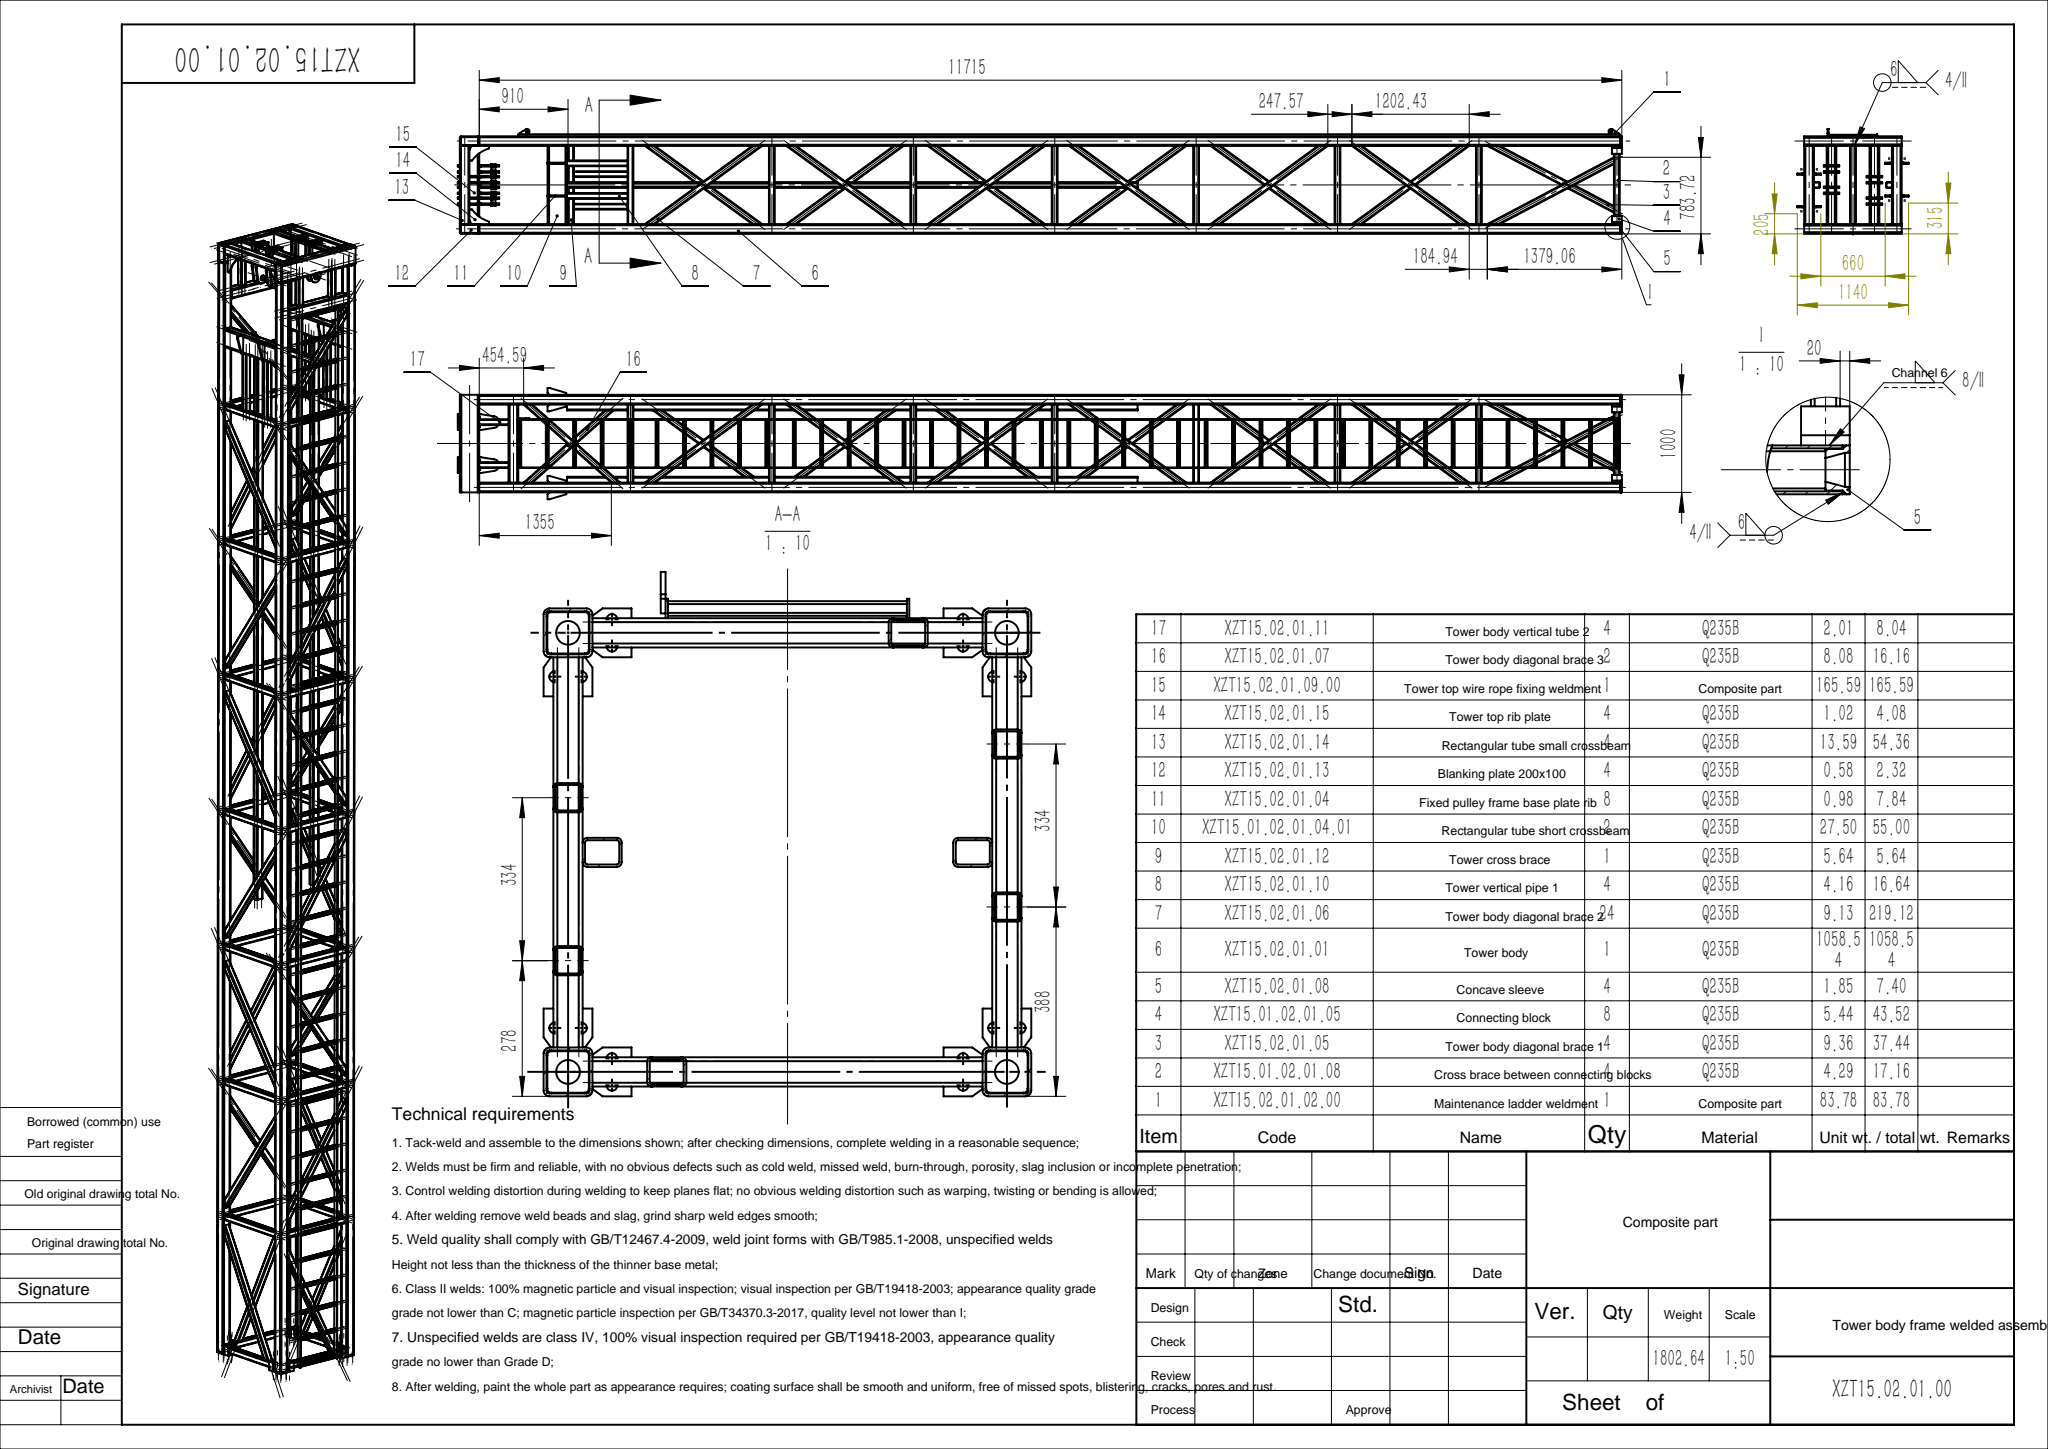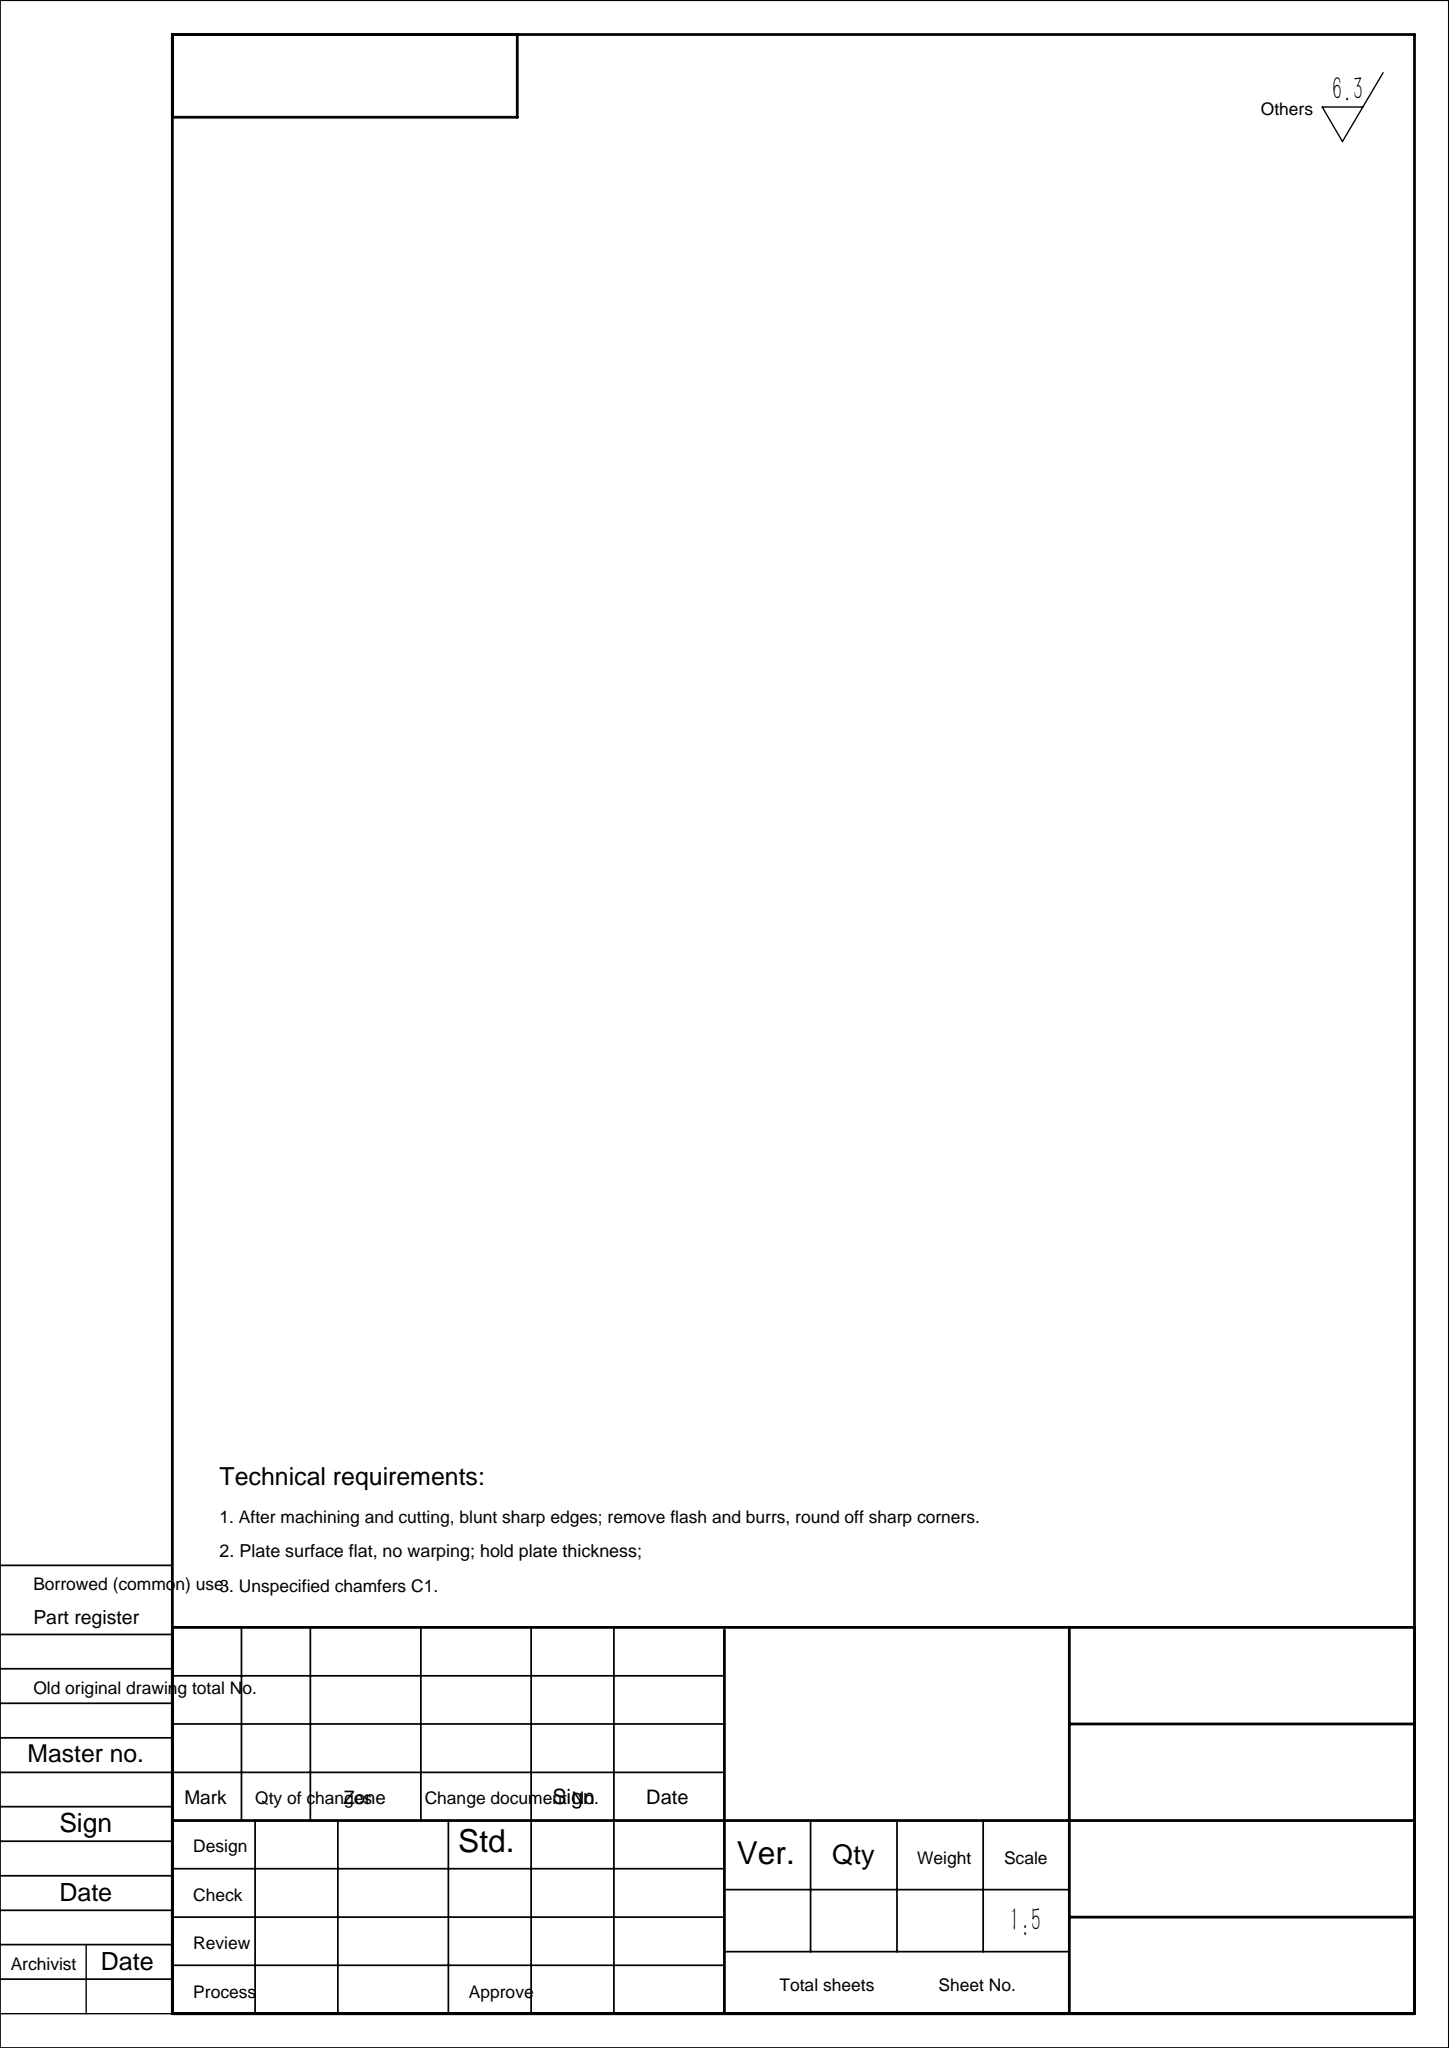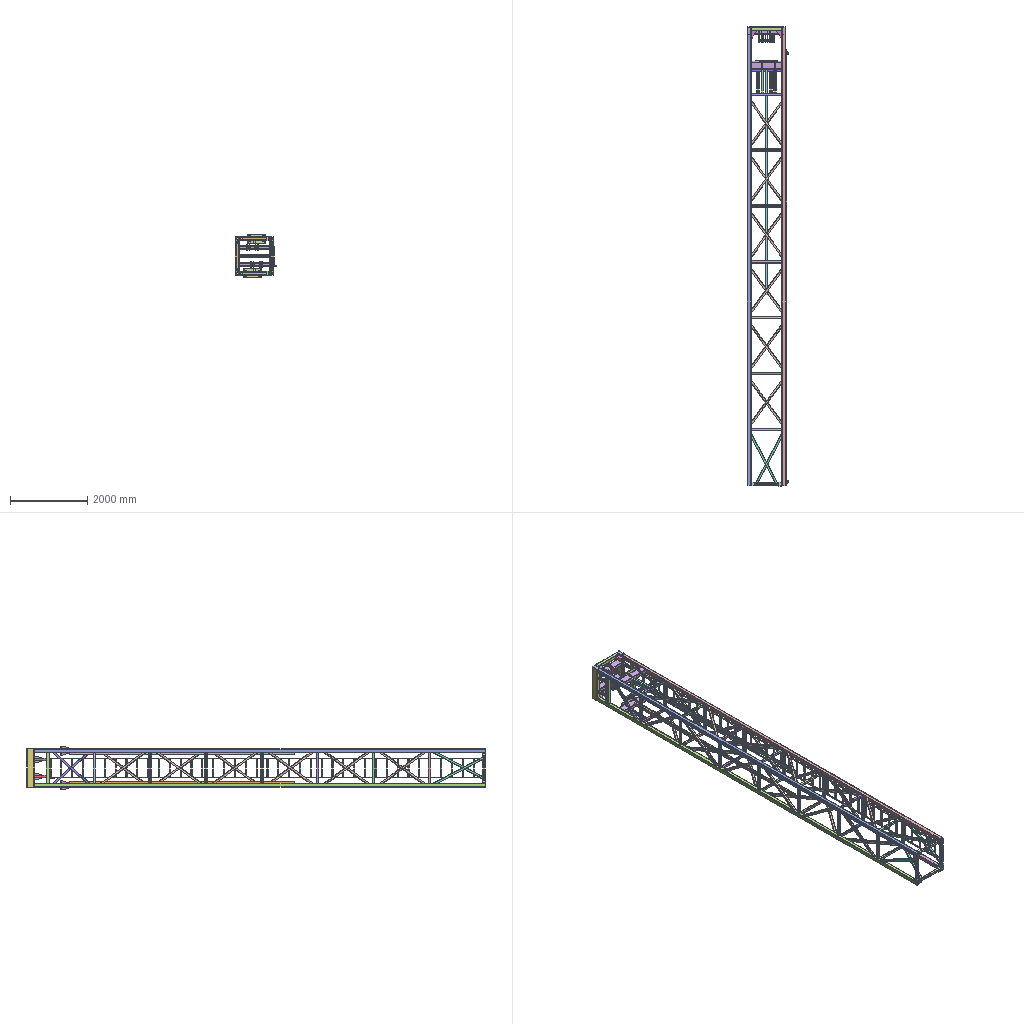Assembly | SolidWorks | 23 different items | 105 placed | box 1075 x 11936 x 1140 mm
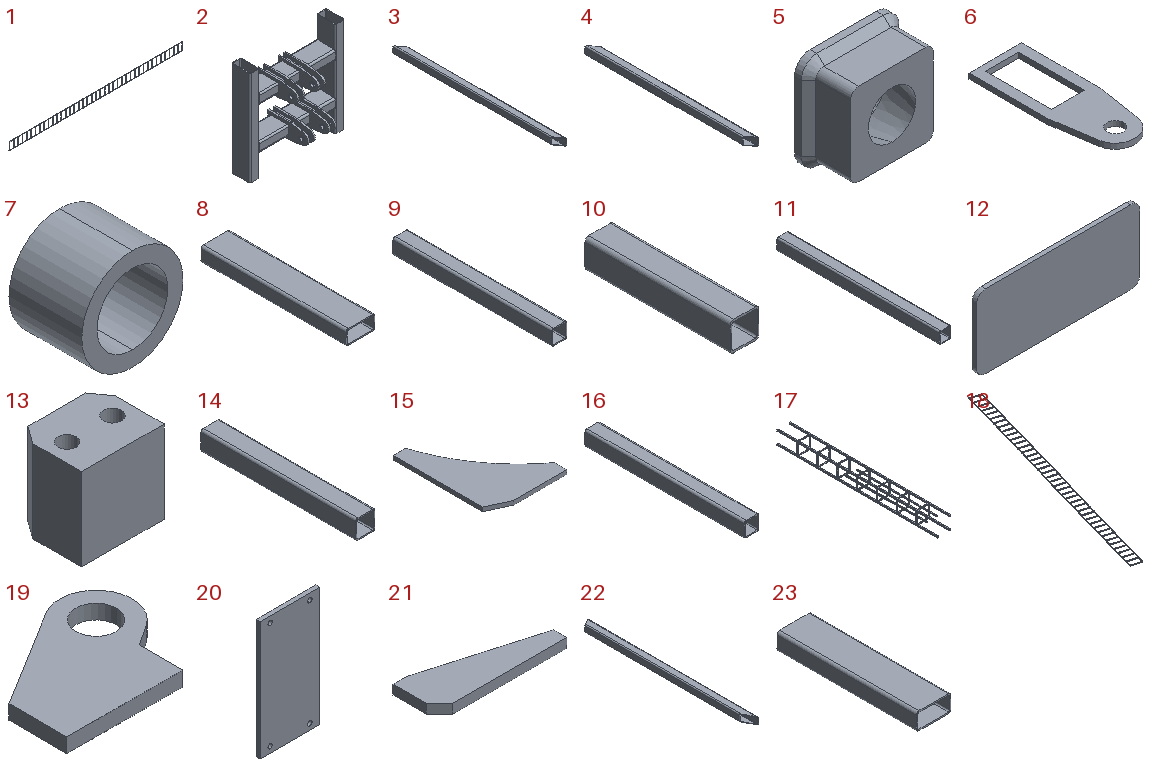Parts list (item | name | quantity | parent item | size | volume | features):
1 | (subassembly) | x1 | - | 11295 x 95 x 510 mm | 10672241 mm3 | features MirrorCompFeat 1, ReferencePattern 1
2 | (subassembly) | x1 | - | 1000 x 425 x 1000 mm | 21094555 mm3 | features MirrorCompFeat 2, ReferencePattern 2
3 | - | x24 | - | 60 x 1443 x 60 mm | 1162925 mm3 | features ICE 1, WeldMemberFeat 1, WeldmentFeature 1
4 | - | x2 | - | 60 x 1272 x 60 mm | 1029576 mm3 | features ICE 1, WeldMemberFeat 1, WeldmentFeature 1
5 | - | x4 | - | 100 x 50 x 100 mm | 236221 mm3 | features Chamfer 1, Extrusion 1, ICE 1, RevCut 1
6 | - | x8 | in 2 | 160 x 425 x 16 mm | 630136 mm3 | features Extrusion 1
7 | - | x8 | in 2 | 50 x 36 x 50 mm | 36050 mm3 | features Extrusion 1
8 | - | x2 | in 2 | 200 x 1000 x 100 mm | 4379186 mm3 | features WeldMemberFeat 1, WeldmentFeature 1
9 | - | x4 | - | 60 x 620 x 60 mm | 529974 mm3 | features WeldMemberFeat 1, WeldmentFeature 1
10 | - | x4 | - | 60 x 300 x 60 mm | 256439 mm3 | features WeldMemberFeat 1, WeldmentFeature 1
11 | - | x1 | - | 60 x 840 x 60 mm | 718029 mm3 | features WeldMemberFeat 1, WeldmentFeature 1
12 | - | x4 | - | 182 x 5 x 82 mm | 74191 mm3 | features Chamfer 1, Extrusion 1, Fillet 1, HoleWzd 1
13 | - | x8 | - | 100 x 80 x 100 mm | 692473 mm3 | features Chamfer 1, Extrusion 1, HoleWzd 1, ICE 1
14 | - | x4 | - | 100 x 800 x 100 mm | 1730634 mm3 | features WeldMemberFeat 1, WeldmentFeature 1
15 | - | x4 | - | 150 x 200 x 8 mm | 129549 mm3 | features Chamfer 1, Extrusion 1, ICE 1
16 | - | x4 | - | 60 x 640 x 60 mm | 547070 mm3 | features WeldMemberFeat 1, WeldmentFeature 1
17 | - | x1 | - | 1000 x 11700 x 1000 mm | 134846254 mm3 | features WeldMemberFeat 3, 3DProfileFeature 1, LPattern 1, WeldCornerFeat 1, WeldmentFeature 1
18 | - | x1 | in 1 | 3594 x 10995 x 40 mm | 10561334 mm3 | features WeldMemberFeat 2, Chamfer 1, ICE 1, LPattern 1, Sweep 1, WeldCornerFeat 1, WeldmentFeature 1
19 | - | x2 | in 1 | 105 x 85 x 10 mm | 55453 mm3 | features Extrusion 1
20 | - | x2 | - | 240 x 16 x 480 mm | 1826914 mm3 | features Chamfer 1, Extrusion 1, Fillet 1, HoleWzd 1
21 | - | x8 | - | 192 x 70 x 14 mm | 125160 mm3 | features Chamfer 1, Extrusion 1
22 | - | x4 | - | 60 x 1468 x 60 mm | 1192621 mm3 | features ICE 1, WeldMemberFeat 1, WeldmentFeature 1
23 | - | x4 | in 2 | 200 x 800 x 100 mm | 3503349 mm3 | features WeldMemberFeat 1, WeldmentFeature 1
Mates (type | each side: item.copy, entity, surface, feature):
In the top assembly
Coincident | 17.1 plane | assembly plane | 4 times
Coincident | 17.1 face plane GB/T 6728-2002 square hollow section 100×100×6(1) | 5.1 face plane Boss-Extrude1 | 2 times
DistanceDim | 5.1 face plane Boss-Extrude1 | 17.1 face plane GB/T 6728-2002 square hollow section 100×100×6(1)
Coincident | 17.1 face plane GB/T 6728-2002 square hollow section 100×100×6(1) | 13.1 face plane Boss-Extrude1 | 2 times
Coincident | 13.1 face plane Boss-Extrude1 | 5.2 face plane Boss-Extrude1
Coincident | 17.1 face plane GB/T 6728-2002 square hollow section 100×100×6(1) | 13.2 face plane Boss-Extrude1 | 2 times
Coincident | 13.1 face plane Boss-Extrude1 | 13.2 face plane Boss-Extrude1
Coincident | 16.1 face plane GB/T 6728-2002 square hollow section 60×60×4(1) | 13.1 face plane Boss-Extrude1
Width | 16.1 face plane GB/T 6728-2002 square hollow section 60×60×4(1) | 16.1 face plane GB/T 6728-2002 square hollow section 60×60×4(1) | 13.1 face plane Boss-Extrude1 | 13.1 face plane Boss-Extrude1 | 2 times
Coincident | 16.1 face plane GB/T 6728-2002 square hollow section 60×60×4(1) | 16.2 face plane GB/T 6728-2002 square hollow section 60×60×4(1)
Coincident | 13.2 face plane Boss-Extrude1 | 16.2 face plane GB/T 6728-2002 square hollow section 60×60×4(1)
Width | 16.2 face plane GB/T 6728-2002 square hollow section 60×60×4(1) | 16.2 face plane GB/T 6728-2002 square hollow section 60×60×4(1) | 13.2 face plane Boss-Extrude1 | 13.2 face plane Boss-Extrude1
Coincident | 17.1 face plane GB/T 6728-2002 square hollow section 100×100×6(1) | 8.1 face plane GB/T 6728-2002 rectangular hollow section 200X100X8(2)
Coincident | 17.1 face plane GB/T 6728-2002 square hollow section 100×100×6(1) | 8.2 face plane GB/T 6728-2002 rectangular hollow section 200X100X8(2) | 2 times
Coincident | 8.2 face plane GB/T 6728-2002 rectangular hollow section 200X100X8(2) | 12.1 face plane Boss-Extrude1
DistanceDim | 12.1 face plane Boss-Extrude1 | 8.2 face plane GB/T 6728-2002 rectangular hollow section 200X100X8(2) | 2 times
Coincident | 8.2 face plane GB/T 6728-2002 rectangular hollow section 200X100X8(2) | 23.1 face plane GB/T 6728-2002 rectangular hollow section 200X100X8(2)
Coincident | 8.1 face plane GB/T 6728-2002 rectangular hollow section 200X100X8(2) | 23.1 face plane GB/T 6728-2002 rectangular hollow section 200X100X8(2)
Coincident | 22.1 face plane Cut-Extrude1 | 16.1 face plane GB/T 6728-2002 square hollow section 60×60×4(1)
Coincident | 22.1 face plane GB/T 6728-2002 square hollow section 60×60×4(1) | 16.1 face plane GB/T 6728-2002 square hollow section 60×60×4(1)
Coincident | 17.1 face plane GB/T 6728-2002 square hollow section 100×100×6(1) | 22.1 face plane Cut-Extrude1
Coincident | 17.1 face plane GB/T 6728-2002 square hollow section 100×100×6(1) | 3.1 face plane Cut-Extrude1
Coincident | 17.1 face plane LinearPattern1 | 3.1 face plane GB/T 6728-2002 square hollow section 60×60×4(1)
Coincident | 17.1 face plane GB/T 6728-2002 square hollow section 100×100×6(1) | 3.2 face plane Cut-Extrude1
Coincident | 17.1 face plane LinearPattern1 | 3.2 face plane GB/T 6728-2002 square hollow section 60×60×4(1)
DistanceDim | 3.1 edge | 17.1 face plane LinearPattern1
DistanceDim | 17.1 face plane LinearPattern1 | 3.2 edge
Coincident | 17.1 face plane GB/T 6728-2002 square hollow section 100×100×6(1) | 4.1 face plane Cut-Extrude1
Coincident | 17.1 face plane GB/T 6728-2002 square hollow section 60×60×4(1) | 4.2 face plane GB/T 6728-2002 square hollow section 60×60×4(1)
Coincident | 17.1 face plane GB/T 6728-2002 square hollow section 100×100×6(1) | 4.2 face plane Cut-Extrude1
Coincident | 17.1 face plane GB/T 6728-2002 square hollow section 60×60×4(1) | 4.1 face plane GB/T 6728-2002 square hollow section 60×60×4(1)
Width | 17.1 face plane GB/T 6728-2002 square hollow section 100×100×6(1) | 17.1 face plane GB/T 6728-2002 square hollow section 100×100×6(1) | 18.1 face plane GB/T 704-1988 hot-rolled flat steel 40×5(1) | 18.1 face plane GB/T 704-1988 hot-rolled flat steel 40×5(1)
Coincident | 17.1 face plane GB/T 6728-2002 square hollow section 60×60×4(1) | 18.1 face plane GB/T 704-1988 hot-rolled flat steel 40×5(1)
Coincident | 17.1 face plane GB/T 6728-2002 square hollow section 60×60×4(1) | 9.1 face plane GB/T 6728-2002 square hollow section 60×60×4(1) | 2 times
Coincident | 9.1 face plane GB/T 6728-2002 square hollow section 60×60×4(1) | 9.2 face plane GB/T 6728-2002 square hollow section 60×60×4(1) | 2 times
DistanceDim | 9.2 face plane GB/T 6728-2002 square hollow section 60×60×4(1) | 9.1 face plane GB/T 6728-2002 square hollow section 60×60×4(1)
DistanceDim | 9.1 face plane GB/T 6728-2002 square hollow section 60×60×4(1) | 17.1 face plane GB/T 6728-2002 square hollow section 100×100×6(1)
Coincident | 9.3 face plane GB/T 6728-2002 square hollow section 60×60×4(1) | 9.4 face plane GB/T 6728-2002 square hollow section 60×60×4(1) | 2 times
DistanceDim | 9.4 face plane GB/T 6728-2002 square hollow section 60×60×4(1) | 9.3 face plane GB/T 6728-2002 square hollow section 60×60×4(1)
Coincident | 17.1 face plane GB/T 6728-2002 square hollow section 60×60×4(1) | 9.3 face plane GB/T 6728-2002 square hollow section 60×60×4(1) | 2 times
DistanceDim | 9.3 face plane GB/T 6728-2002 square hollow section 60×60×4(1) | 17.1 face plane GB/T 6728-2002 square hollow section 100×100×6(1)
DistanceDim | 20.1 face plane Boss-Extrude1 | 17.1 face plane GB/T 6728-2002 square hollow section 100×100×6(1) | 2 times
Coincident | 20.1 face plane Boss-Extrude1 | 20.2 face plane Boss-Extrude1
DistanceDim | 20.2 face plane Boss-Extrude1 | 17.1 face plane GB/T 6728-2002 square hollow section 100×100×6(1) | 2 times
Coincident | 8.1 face plane GB/T 6728-2002 rectangular hollow section 200X100X8(2) | 14.1 face plane GB/T 6728-2002 square hollow section 100×100×6(1)
Coincident | 8.2 face plane GB/T 6728-2002 rectangular hollow section 200X100X8(2) | 14.1 face plane GB/T 6728-2002 square hollow section 100×100×6(1) | 2 times
DistanceDim | 4.1 edge | 8.2 face plane GB/T 6728-2002 rectangular hollow section 200X100X8(2)
DistanceDim | 4.2 edge | 8.1 face plane GB/T 6728-2002 rectangular hollow section 200X100X8(2)
Coincident | 9.1 face plane GB/T 6728-2002 square hollow section 60×60×4(1) | 23.1 face plane GB/T 6728-2002 rectangular hollow section 200X100X8(2)
Coincident | 20.1 face plane Boss-Extrude1 | 23.1 face plane GB/T 6728-2002 rectangular hollow section 200X100X8(2)
Coincident | 10.1 face plane GB/T 6728-2002 square hollow section 60×60×4(1) | 14.2 face plane GB/T 6728-2002 square hollow section 100×100×6(1)
Coincident | 17.1 face plane GB/T 6728-2002 square hollow section 100×100×6(1) | 14.2 face plane GB/T 6728-2002 square hollow section 100×100×6(1) | 2 times
Coincident | 8.1 face plane GB/T 6728-2002 rectangular hollow section 200X100X8(2) | 10.1 face plane GB/T 6728-2002 square hollow section 60×60×4(1)
DistanceDim | 10.1 face plane GB/T 6728-2002 square hollow section 60×60×4(1) | 10.2 face plane GB/T 6728-2002 square hollow section 60×60×4(1)
Coincident | 21.1 face plane Boss-Extrude1 | 23.1 face plane GB/T 6728-2002 rectangular hollow section 200X100X8(2)
Coincident | 20.1 face plane Boss-Extrude1 | 21.1 face plane Boss-Extrude1
Width | 21.1 face plane Boss-Extrude1 | 21.1 face plane Boss-Extrude1 | 9.1 face plane GB/T 6728-2002 square hollow section 60×60×4(1) | 9.1 face plane GB/T 6728-2002 square hollow section 60×60×4(1)
Coincident | 21.1 face plane Boss-Extrude1 | 21.2 face plane Boss-Extrude1 | 2 times
Width | 9.2 face plane GB/T 6728-2002 square hollow section 60×60×4(1) | 9.2 face plane GB/T 6728-2002 square hollow section 60×60×4(1) | 21.2 face plane Boss-Extrude1 | 21.2 face plane Boss-Extrude1
Coincident | 21.3 face plane Boss-Extrude1 | 21.4 face plane Boss-Extrude1 | 2 times
Coincident | 20.2 face plane Boss-Extrude1 | 21.3 face plane Boss-Extrude1
Coincident | 23.2 face plane GB/T 6728-2002 rectangular hollow section 200X100X8(2) | 21.3 face plane Boss-Extrude1
Width | 21.3 face plane Boss-Extrude1 | 21.3 face plane Boss-Extrude1 | 9.4 face plane GB/T 6728-2002 square hollow section 60×60×4(1) | 9.4 face plane GB/T 6728-2002 square hollow section 60×60×4(1)
DistanceDim | 21.4 face plane Boss-Extrude1 | 21.3 face plane Boss-Extrude1
Coincident | 21.5 face plane Boss-Extrude1 | 21.6 face plane Boss-Extrude1 | 2 times
DistanceDim | 21.6 face plane Boss-Extrude1 | 21.5 face plane Boss-Extrude1
Coincident | 21.3 face plane Boss-Extrude1 | 21.6 face plane Boss-Extrude1 | 2 times
Coincident | 23.2 face plane GB/T 6728-2002 rectangular hollow section 200X100X8(2) | 21.6 face plane Boss-Extrude1
Coincident | 21.7 face plane Boss-Extrude1 | 21.8 face plane Boss-Extrude1 | 2 times
DistanceDim | 21.8 face plane Boss-Extrude1 | 21.7 face plane Boss-Extrude1
Coincident | 23.1 face plane GB/T 6728-2002 rectangular hollow section 200X100X8(2) | 21.7 face plane Boss-Extrude1
Coincident | 21.2 face plane Boss-Extrude1 | 21.7 face plane Boss-Extrude1 | 2 times
Coincident | 14.1 face plane GB/T 6728-2002 square hollow section 100×100×6(1) | 15.1 face plane Boss-Extrude1
Coincident | 17.1 face plane GB/T 6728-2002 square hollow section 100×100×6(1) | 15.1 face plane Boss-Extrude1
Width | 15.1 face plane Boss-Extrude1 | 15.1 face plane Boss-Extrude1 | 14.1 face plane GB/T 6728-2002 square hollow section 100×100×6(1) | 14.1 face plane GB/T 6728-2002 square hollow section 100×100×6(1)
Coincident | 18.1 face plane GB/T 6728-2002 square hollow section 30×3-example.com(1) | 14.2 face plane GB/T 6728-2002 square hollow section 100×100×6(1)
Width | 14.2 face plane GB/T 6728-2002 square hollow section 100×100×6(1) | 14.2 face plane GB/T 6728-2002 square hollow section 100×100×6(1) | 10.1 face plane GB/T 6728-2002 square hollow section 60×60×4(1) | 10.1 face plane GB/T 6728-2002 square hollow section 60×60×4(1)
Coincident | 4.1 face plane GB/T 6728-2002 square hollow section 60×60×4(1) | 11.1 face plane GB/T 6728-2002 square hollow section 60×60×4(1)
Coincident | 11.1 plane | assembly plane
DistanceDim | 18.1 face plane LinearPattern1 | 11.1 face plane GB/T 6728-2002 square hollow section 60×60×4(1)
In subassembly 1
Coincident | 18.2 face plane GB/T 704-1988 hot-rolled flat steel 40×5(1) | 1.1 plane | 2 times
Symmetric | 18.2 face plane GB/T 704-1988 hot-rolled flat steel 40×5(1) | 18.2 face plane GB/T 704-1988 hot-rolled flat steel 40×5(1) | 1.1 plane
Coincident | 18.2 face plane GB/T 704-1988 hot-rolled flat steel 40×5(1) | 19.1 face plane Boss-Extrude1
DistanceDim | 19.1 face plane Boss-Extrude1 | 18.2 face plane GB/T 704-1988 hot-rolled flat steel 40×5(1)
DistanceDim | 18.2 face plane GB/T 704-1988 hot-rolled flat steel 40×5(1) | 19.1 face plane Boss-Extrude1
In subassembly 2
Symmetric | 8.3 face plane GB/T 6728-2002 rectangular hollow section 200X100X8(2) | 8.3 face plane GB/T 6728-2002 rectangular hollow section 200X100X8(2) | 2.1 plane
Coincident | 8.3 plane | 2.1 plane
DistanceDim | 8.3 face plane GB/T 6728-2002 rectangular hollow section 200X100X8(2) | 8.4 face plane GB/T 6728-2002 rectangular hollow section 200X100X8(2)
Coincident | 23.1 face plane GB/T 6728-2002 rectangular hollow section 200X100X8(2) | 8.4 face plane GB/T 6728-2002 rectangular hollow section 200X100X8(2) | 2 times
DistanceDim | 23.1 face plane GB/T 6728-2002 rectangular hollow section 200X100X8(2) | 23.2 face plane GB/T 6728-2002 rectangular hollow section 200X100X8(2)
Coincident | 6.1 face plane Boss-Extrude1 | 6.2 face plane Boss-Extrude1 | 2 times
DistanceDim | 6.1 face plane Boss-Extrude1 | 6.2 face plane Boss-Extrude1
Concentric | 6.1 face cylinder Boss-Extrude1 | 7.1 face cylinder Boss-Extrude1
Width | 7.1 face plane Boss-Extrude1 | 7.1 face plane Boss-Extrude1 | 6.1 face plane Boss-Extrude1 | 6.1 face plane Boss-Extrude1
Concentric | 6.2 face cylinder Boss-Extrude1 | 7.2 face cylinder Boss-Extrude1
Width | 7.2 face plane Boss-Extrude1 | 7.2 face plane Boss-Extrude1 | 6.2 face plane Boss-Extrude1 | 6.2 face plane Boss-Extrude1
Width | 6.2 face plane Boss-Extrude1 | 6.2 face plane Boss-Extrude1 | 23.1 face plane GB/T 6728-2002 rectangular hollow section 200X100X8(2) | 23.1 face plane GB/T 6728-2002 rectangular hollow section 200X100X8(2) | 2 times
Coincident | 6.3 face plane Boss-Extrude1 | 6.4 face plane Boss-Extrude1 | 2 times
Concentric | 7.3 face cylinder Boss-Extrude1 | 6.4 face cylinder Boss-Extrude1
Width | 7.3 face plane Boss-Extrude1 | 7.3 face plane Boss-Extrude1 | 6.4 face plane Boss-Extrude1 | 6.4 face plane Boss-Extrude1
DistanceDim | 6.4 face plane Boss-Extrude1 | 6.3 face plane Boss-Extrude1
Width | 7.4 face plane Boss-Extrude1 | 7.4 face plane Boss-Extrude1 | 6.3 face plane Boss-Extrude1 | 6.3 face plane Boss-Extrude1
Concentric | 6.3 face cylinder Boss-Extrude1 | 7.4 face cylinder Boss-Extrude1
Coincident | 6.1 face plane Boss-Extrude1 | 6.3 face plane Boss-Extrude1 | 2 times
DistanceDim | 6.2 face plane Boss-Extrude1 | 8.3 face plane GB/T 6728-2002 rectangular hollow section 200X100X8(2)
DistanceDim | 6.3 face plane Boss-Extrude1 | 6.1 face plane Boss-Extrude1
Coincident | 6.5 face plane Boss-Extrude1 | 6.6 face plane Boss-Extrude1 | 2 times
Concentric | 7.5 face cylinder Boss-Extrude1 | 6.5 face cylinder Boss-Extrude1
Width | 7.5 face plane Boss-Extrude1 | 7.5 face plane Boss-Extrude1 | 6.5 face plane Boss-Extrude1 | 6.5 face plane Boss-Extrude1
Coincident | 6.5 face plane Boss-Extrude1 | 6.7 face plane Boss-Extrude1 | 2 times
Coincident | 6.7 face plane Boss-Extrude1 | 6.8 face plane Boss-Extrude1 | 2 times
DistanceDim | 6.5 face plane Boss-Extrude1 | 6.6 face plane Boss-Extrude1
Width | 7.6 face plane Boss-Extrude1 | 7.6 face plane Boss-Extrude1 | 6.6 face plane Boss-Extrude1 | 6.6 face plane Boss-Extrude1
DistanceDim | 6.8 face plane Boss-Extrude1 | 6.7 face plane Boss-Extrude1
Concentric | 6.6 face cylinder Boss-Extrude1 | 7.6 face cylinder Boss-Extrude1
Concentric | 7.7 face cylinder Boss-Extrude1 | 6.8 face cylinder Boss-Extrude1
Width | 7.8 face plane Boss-Extrude1 | 7.8 face plane Boss-Extrude1 | 6.7 face plane Boss-Extrude1 | 6.7 face plane Boss-Extrude1
DistanceDim | 6.7 face plane Boss-Extrude1 | 6.5 face plane Boss-Extrude1
Width | 7.7 face plane Boss-Extrude1 | 7.7 face plane Boss-Extrude1 | 6.8 face plane Boss-Extrude1 | 6.8 face plane Boss-Extrude1
Concentric | 6.7 face cylinder Boss-Extrude1 | 7.8 face cylinder Boss-Extrude1
Coincident | 6.1 face plane Boss-Extrude1 | 6.5 face plane Boss-Extrude1
Width | 6.6 face plane Boss-Extrude1 | 6.6 face plane Boss-Extrude1 | 23.2 face plane GB/T 6728-2002 rectangular hollow section 200X100X8(2) | 23.2 face plane GB/T 6728-2002 rectangular hollow section 200X100X8(2)
DistanceDim | 6.6 face plane Boss-Extrude1 | 8.3 face plane GB/T 6728-2002 rectangular hollow section 200X100X8(2)